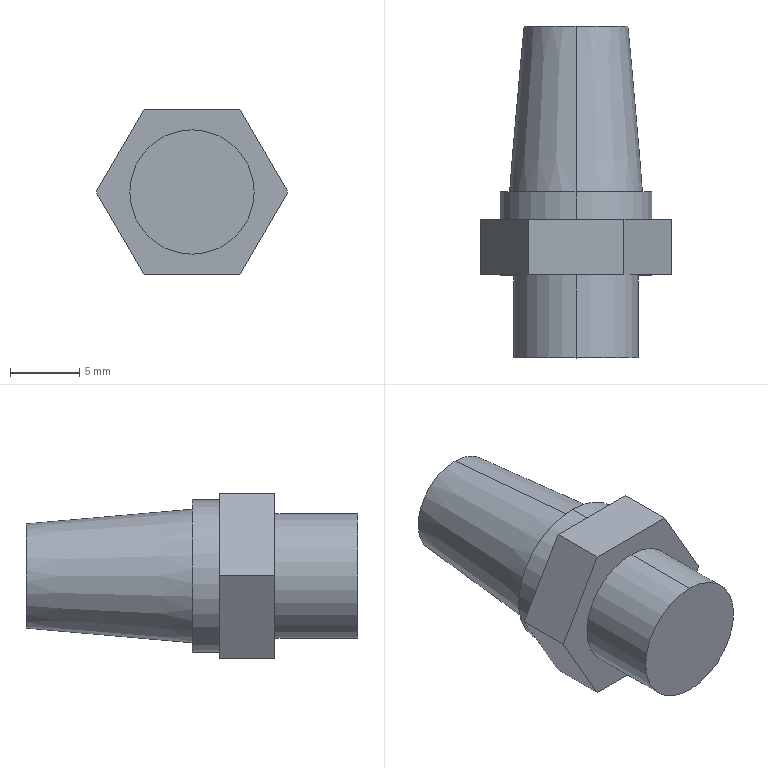Part | STEP file | Universal Copper Muffler BSL-01 | 1 solid | 17 faces | box 13.856 x 24 x 12 mm | volume 1771 mm3 | plane 11 | cylinder 4 | cone 2 | commonest cylinder face diameters 9 x2 11 x2
STEP:
#1=CARTESIAN_POINT('',(0.,0.,0.));
#2=DIRECTION('',(0.,0.,1.));
#3=DIRECTION('',(1.,0.,0.));
#4=AXIS2_PLACEMENT_3D('',#1,#2,#3);
#5=CARTESIAN_POINT('',(0.,24.,3.775));
#6=VERTEX_POINT('',#5);
#7=CARTESIAN_POINT('',(0.,24.,-3.775));
#8=VERTEX_POINT('',#7);
#9=CARTESIAN_POINT('',(0.,24.,0.));
#10=DIRECTION('',(0.,1.,0.));
#11=DIRECTION('',(0.,0.,1.));
#12=AXIS2_PLACEMENT_3D('',#9,#10,#11);
#13=CIRCLE('',#12,3.775);
#14=CARTESIAN_POINT('',(0.,24.,0.));
#15=DIRECTION('',(0.,-1.,0.));
#16=DIRECTION('',(0.,0.,-1.));
#17=AXIS2_PLACEMENT_3D('',#14,#15,#16);
#18=CONICAL_SURFACE('',#17,3.775,0.08727);
#19=CARTESIAN_POINT('',(3.142,0.));
#20=DIRECTION('',(-1.,0.));
#21=VECTOR('',#20,1.);
#22=LINE('',#19,#21);
#23=(GEOMETRIC_REPRESENTATION_CONTEXT(2)PARAMETRIC_REPRESENTATION_CONTEXT()REPRESENTATION_CONTEXT('',''));
#24=DEFINITIONAL_REPRESENTATION('',(#22),#23);
#25=PCURVE('',#18,#24);
#26=CARTESIAN_POINT('',(0.,24.,0.));
#27=DIRECTION('',(0.,1.,0.));
#28=DIRECTION('',(0.,0.,1.));
#29=AXIS2_PLACEMENT_3D('',#26,#27,#28);
#30=PLANE('',#29);
#31=CARTESIAN_POINT('',(0.,0.));
#32=DIRECTION('',(1.,0.));
#33=AXIS2_PLACEMENT_2D('',#31,#32);
#34=CIRCLE('',#33,3.775);
#35=(GEOMETRIC_REPRESENTATION_CONTEXT(2)PARAMETRIC_REPRESENTATION_CONTEXT()REPRESENTATION_CONTEXT('',''));
#36=DEFINITIONAL_REPRESENTATION('',(#34),#35);
#37=PCURVE('',#30,#36);
#38=SURFACE_CURVE('',#13,(#25,#37),.PCURVE_S1.);
#39=EDGE_CURVE('',#6,#8,#38,.T.);
#40=ORIENTED_EDGE('',*,*,#39,.F.);
#41=CARTESIAN_POINT('',(0.,12.,4.825));
#42=VERTEX_POINT('',#41);
#43=CARTESIAN_POINT('',(0.,24.,3.775));
#44=DIRECTION('',(0.,-0.9962,0.08716));
#45=VECTOR('',#44,1.);
#46=LINE('',#43,#45);
#47=CARTESIAN_POINT('',(3.142,0.));
#48=DIRECTION('',(0.,1.));
#49=VECTOR('',#48,1.);
#50=LINE('',#47,#49);
#51=(GEOMETRIC_REPRESENTATION_CONTEXT(2)PARAMETRIC_REPRESENTATION_CONTEXT()REPRESENTATION_CONTEXT('',''));
#52=DEFINITIONAL_REPRESENTATION('',(#50),#51);
#53=PCURVE('',#18,#52);
#54=CARTESIAN_POINT('',(0.,24.,0.));
#55=DIRECTION('',(0.,-1.,0.));
#56=DIRECTION('',(0.,0.,-1.));
#57=AXIS2_PLACEMENT_3D('',#54,#55,#56);
#58=CONICAL_SURFACE('',#57,3.775,0.08727);
#59=CARTESIAN_POINT('',(3.142,0.));
#60=DIRECTION('',(0.,1.));
#61=VECTOR('',#60,1.);
#62=LINE('',#59,#61);
#63=(GEOMETRIC_REPRESENTATION_CONTEXT(2)PARAMETRIC_REPRESENTATION_CONTEXT()REPRESENTATION_CONTEXT('',''));
#64=DEFINITIONAL_REPRESENTATION('',(#62),#63);
#65=PCURVE('',#58,#64);
#66=SURFACE_CURVE('',#46,(#53,#65),.PCURVE_S1.);
#67=EDGE_CURVE('',#6,#42,#66,.T.);
#68=ORIENTED_EDGE('',*,*,#67,.T.);
#69=CARTESIAN_POINT('',(0.,12.,-4.825));
#70=VERTEX_POINT('',#69);
#71=CARTESIAN_POINT('',(0.,12.,0.));
#72=DIRECTION('',(0.,-1.,0.));
#73=DIRECTION('',(0.,0.,1.));
#74=AXIS2_PLACEMENT_3D('',#71,#72,#73);
#75=CIRCLE('',#74,4.825);
#76=CARTESIAN_POINT('',(-3.142,12.));
#77=DIRECTION('',(1.,0.));
#78=VECTOR('',#77,1.);
#79=LINE('',#76,#78);
#80=(GEOMETRIC_REPRESENTATION_CONTEXT(2)PARAMETRIC_REPRESENTATION_CONTEXT()REPRESENTATION_CONTEXT('',''));
#81=DEFINITIONAL_REPRESENTATION('',(#79),#80);
#82=PCURVE('',#18,#81);
#83=CARTESIAN_POINT('',(0.,12.,0.));
#84=DIRECTION('',(0.,1.,0.));
#85=DIRECTION('',(0.,0.,1.));
#86=AXIS2_PLACEMENT_3D('',#83,#84,#85);
#87=PLANE('',#86);
#88=CARTESIAN_POINT('',(4.825,0.));
#89=CARTESIAN_POINT('',(4.825,-8.357));
#90=CARTESIAN_POINT('',(-2.413,-4.179));
#91=CARTESIAN_POINT('',(-9.65,0.));
#92=CARTESIAN_POINT('',(-2.413,4.179));
#93=CARTESIAN_POINT('',(4.825,8.357));
#94=CARTESIAN_POINT('',(4.825,0.));
#95=(BOUNDED_CURVE()B_SPLINE_CURVE(2,(#88,#89,#90,#91,#92,#93,#94),.UNSPECIFIED.,.T.,.F.)B_SPLINE_CURVE_WITH_KNOTS((1,2,2,2,2,1),(-2.094,0.,2.094,4.189,6.283,8.378),.UNSPECIFIED.)CURVE()GEOMETRIC_REPRESENTATION_ITEM()RATIONAL_B_SPLINE_CURVE((1.,0.5,1.,0.5,1.,0.5,1.))REPRESENTATION_ITEM(''));
#96=(GEOMETRIC_REPRESENTATION_CONTEXT(2)PARAMETRIC_REPRESENTATION_CONTEXT()REPRESENTATION_CONTEXT('',''));
#97=DEFINITIONAL_REPRESENTATION('',(#95),#96);
#98=PCURVE('',#87,#97);
#99=SURFACE_CURVE('',#75,(#82,#98),.PCURVE_S1.);
#100=EDGE_CURVE('',#70,#42,#99,.T.);
#101=ORIENTED_EDGE('',*,*,#100,.F.);
#102=CARTESIAN_POINT('',(0.,24.,-3.775));
#103=DIRECTION('',(0.,-0.9962,-0.08716));
#104=VECTOR('',#103,1.);
#105=LINE('',#102,#104);
#106=CARTESIAN_POINT('',(0.,0.));
#107=DIRECTION('',(0.,1.));
#108=VECTOR('',#107,1.);
#109=LINE('',#106,#108);
#110=(GEOMETRIC_REPRESENTATION_CONTEXT(2)PARAMETRIC_REPRESENTATION_CONTEXT()REPRESENTATION_CONTEXT('',''));
#111=DEFINITIONAL_REPRESENTATION('',(#109),#110);
#112=PCURVE('',#18,#111);
#113=CARTESIAN_POINT('',(6.283,0.));
#114=DIRECTION('',(0.,1.));
#115=VECTOR('',#114,1.);
#116=LINE('',#113,#115);
#117=(GEOMETRIC_REPRESENTATION_CONTEXT(2)PARAMETRIC_REPRESENTATION_CONTEXT()REPRESENTATION_CONTEXT('',''));
#118=DEFINITIONAL_REPRESENTATION('',(#116),#117);
#119=PCURVE('',#58,#118);
#120=SURFACE_CURVE('',#105,(#112,#119),.PCURVE_S1.);
#121=EDGE_CURVE('',#8,#70,#120,.T.);
#122=ORIENTED_EDGE('',*,*,#121,.F.);
#123=EDGE_LOOP('',(#40,#68,#101,#122));
#124=FACE_BOUND('',#123,.T.);
#125=ADVANCED_FACE('',(#124),#18,.T.);
#126=CARTESIAN_POINT('',(0.,12.,5.5));
#127=VERTEX_POINT('',#126);
#128=CARTESIAN_POINT('',(0.,12.,-5.5));
#129=VERTEX_POINT('',#128);
#130=CARTESIAN_POINT('',(0.,12.,0.));
#131=DIRECTION('',(0.,1.,0.));
#132=DIRECTION('',(0.,0.,1.));
#133=AXIS2_PLACEMENT_3D('',#130,#131,#132);
#134=CIRCLE('',#133,5.5);
#135=CARTESIAN_POINT('',(0.,12.,0.));
#136=DIRECTION('',(0.,-1.,0.));
#137=DIRECTION('',(0.,0.,-1.));
#138=AXIS2_PLACEMENT_3D('',#135,#136,#137);
#139=CYLINDRICAL_SURFACE('',#138,5.5);
#140=CARTESIAN_POINT('',(3.142,0.));
#141=DIRECTION('',(-1.,0.));
#142=VECTOR('',#141,1.);
#143=LINE('',#140,#142);
#144=(GEOMETRIC_REPRESENTATION_CONTEXT(2)PARAMETRIC_REPRESENTATION_CONTEXT()REPRESENTATION_CONTEXT('',''));
#145=DEFINITIONAL_REPRESENTATION('',(#143),#144);
#146=PCURVE('',#139,#145);
#147=CARTESIAN_POINT('',(0.,0.));
#148=DIRECTION('',(1.,0.));
#149=AXIS2_PLACEMENT_2D('',#147,#148);
#150=CIRCLE('',#149,5.5);
#151=(GEOMETRIC_REPRESENTATION_CONTEXT(2)PARAMETRIC_REPRESENTATION_CONTEXT()REPRESENTATION_CONTEXT('',''));
#152=DEFINITIONAL_REPRESENTATION('',(#150),#151);
#153=PCURVE('',#87,#152);
#154=SURFACE_CURVE('',#134,(#146,#153),.PCURVE_S1.);
#155=EDGE_CURVE('',#127,#129,#154,.T.);
#156=ORIENTED_EDGE('',*,*,#155,.F.);
#157=CARTESIAN_POINT('',(0.,10.,5.5));
#158=VERTEX_POINT('',#157);
#159=CARTESIAN_POINT('',(0.,12.,5.5));
#160=DIRECTION('',(0.,-1.,0.));
#161=VECTOR('',#160,1.);
#162=LINE('',#159,#161);
#163=CARTESIAN_POINT('',(3.142,0.));
#164=DIRECTION('',(0.,1.));
#165=VECTOR('',#164,1.);
#166=LINE('',#163,#165);
#167=(GEOMETRIC_REPRESENTATION_CONTEXT(2)PARAMETRIC_REPRESENTATION_CONTEXT()REPRESENTATION_CONTEXT('',''));
#168=DEFINITIONAL_REPRESENTATION('',(#166),#167);
#169=PCURVE('',#139,#168);
#170=CARTESIAN_POINT('',(0.,12.,0.));
#171=DIRECTION('',(0.,-1.,0.));
#172=DIRECTION('',(0.,0.,-1.));
#173=AXIS2_PLACEMENT_3D('',#170,#171,#172);
#174=CYLINDRICAL_SURFACE('',#173,5.5);
#175=CARTESIAN_POINT('',(3.142,0.));
#176=DIRECTION('',(0.,1.));
#177=VECTOR('',#176,1.);
#178=LINE('',#175,#177);
#179=(GEOMETRIC_REPRESENTATION_CONTEXT(2)PARAMETRIC_REPRESENTATION_CONTEXT()REPRESENTATION_CONTEXT('',''));
#180=DEFINITIONAL_REPRESENTATION('',(#178),#179);
#181=PCURVE('',#174,#180);
#182=SURFACE_CURVE('',#162,(#169,#181),.PCURVE_S1.);
#183=EDGE_CURVE('',#127,#158,#182,.T.);
#184=ORIENTED_EDGE('',*,*,#183,.T.);
#185=CARTESIAN_POINT('',(0.,10.,-5.5));
#186=VERTEX_POINT('',#185);
#187=CARTESIAN_POINT('',(0.,10.,0.));
#188=DIRECTION('',(0.,1.,0.));
#189=DIRECTION('',(0.,0.,1.));
#190=AXIS2_PLACEMENT_3D('',#187,#188,#189);
#191=CIRCLE('',#190,5.5);
#192=CARTESIAN_POINT('',(3.142,2.));
#193=DIRECTION('',(-1.,0.));
#194=VECTOR('',#193,1.);
#195=LINE('',#192,#194);
#196=(GEOMETRIC_REPRESENTATION_CONTEXT(2)PARAMETRIC_REPRESENTATION_CONTEXT()REPRESENTATION_CONTEXT('',''));
#197=DEFINITIONAL_REPRESENTATION('',(#195),#196);
#198=PCURVE('',#139,#197);
#199=CARTESIAN_POINT('',(0.,10.,0.));
#200=DIRECTION('',(0.,1.,0.));
#201=DIRECTION('',(0.,0.,1.));
#202=AXIS2_PLACEMENT_3D('',#199,#200,#201);
#203=PLANE('',#202);
#204=CARTESIAN_POINT('',(0.,0.));
#205=DIRECTION('',(1.,0.));
#206=AXIS2_PLACEMENT_2D('',#204,#205);
#207=CIRCLE('',#206,5.5);
#208=(GEOMETRIC_REPRESENTATION_CONTEXT(2)PARAMETRIC_REPRESENTATION_CONTEXT()REPRESENTATION_CONTEXT('',''));
#209=DEFINITIONAL_REPRESENTATION('',(#207),#208);
#210=PCURVE('',#203,#209);
#211=SURFACE_CURVE('',#191,(#198,#210),.PCURVE_S1.);
#212=EDGE_CURVE('',#158,#186,#211,.T.);
#213=ORIENTED_EDGE('',*,*,#212,.T.);
#214=CARTESIAN_POINT('',(0.,12.,-5.5));
#215=DIRECTION('',(0.,-1.,0.));
#216=VECTOR('',#215,1.);
#217=LINE('',#214,#216);
#218=CARTESIAN_POINT('',(0.,0.));
#219=DIRECTION('',(0.,1.));
#220=VECTOR('',#219,1.);
#221=LINE('',#218,#220);
#222=(GEOMETRIC_REPRESENTATION_CONTEXT(2)PARAMETRIC_REPRESENTATION_CONTEXT()REPRESENTATION_CONTEXT('',''));
#223=DEFINITIONAL_REPRESENTATION('',(#221),#222);
#224=PCURVE('',#139,#223);
#225=CARTESIAN_POINT('',(6.283,0.));
#226=DIRECTION('',(0.,1.));
#227=VECTOR('',#226,1.);
#228=LINE('',#225,#227);
#229=(GEOMETRIC_REPRESENTATION_CONTEXT(2)PARAMETRIC_REPRESENTATION_CONTEXT()REPRESENTATION_CONTEXT('',''));
#230=DEFINITIONAL_REPRESENTATION('',(#228),#229);
#231=PCURVE('',#174,#230);
#232=SURFACE_CURVE('',#217,(#224,#231),.PCURVE_S1.);
#233=EDGE_CURVE('',#129,#186,#232,.T.);
#234=ORIENTED_EDGE('',*,*,#233,.F.);
#235=EDGE_LOOP('',(#156,#184,#213,#234));
#236=FACE_BOUND('',#235,.T.);
#237=ADVANCED_FACE('',(#236),#139,.T.);
#238=CARTESIAN_POINT('',(0.,6.,4.5));
#239=VERTEX_POINT('',#238);
#240=CARTESIAN_POINT('',(0.,6.,-4.5));
#241=VERTEX_POINT('',#240);
#242=CARTESIAN_POINT('',(0.,6.,0.));
#243=DIRECTION('',(0.,1.,0.));
#244=DIRECTION('',(0.,0.,1.));
#245=AXIS2_PLACEMENT_3D('',#242,#243,#244);
#246=CIRCLE('',#245,4.5);
#247=CARTESIAN_POINT('',(0.,6.,0.));
#248=DIRECTION('',(0.,-1.,0.));
#249=DIRECTION('',(0.,0.,-1.));
#250=AXIS2_PLACEMENT_3D('',#247,#248,#249);
#251=CYLINDRICAL_SURFACE('',#250,4.5);
#252=CARTESIAN_POINT('',(3.142,0.));
#253=DIRECTION('',(-1.,0.));
#254=VECTOR('',#253,1.);
#255=LINE('',#252,#254);
#256=(GEOMETRIC_REPRESENTATION_CONTEXT(2)PARAMETRIC_REPRESENTATION_CONTEXT()REPRESENTATION_CONTEXT('',''));
#257=DEFINITIONAL_REPRESENTATION('',(#255),#256);
#258=PCURVE('',#251,#257);
#259=CARTESIAN_POINT('',(0.,6.,0.));
#260=DIRECTION('',(0.,1.,0.));
#261=DIRECTION('',(0.,0.,1.));
#262=AXIS2_PLACEMENT_3D('',#259,#260,#261);
#263=PLANE('',#262);
#264=CARTESIAN_POINT('',(0.,0.));
#265=DIRECTION('',(1.,0.));
#266=AXIS2_PLACEMENT_2D('',#264,#265);
#267=CIRCLE('',#266,4.5);
#268=(GEOMETRIC_REPRESENTATION_CONTEXT(2)PARAMETRIC_REPRESENTATION_CONTEXT()REPRESENTATION_CONTEXT('',''));
#269=DEFINITIONAL_REPRESENTATION('',(#267),#268);
#270=PCURVE('',#263,#269);
#271=SURFACE_CURVE('',#246,(#258,#270),.PCURVE_S1.);
#272=EDGE_CURVE('',#239,#241,#271,.T.);
#273=ORIENTED_EDGE('',*,*,#272,.F.);
#274=CARTESIAN_POINT('',(0.,0.,4.5));
#275=VERTEX_POINT('',#274);
#276=CARTESIAN_POINT('',(0.,6.,4.5));
#277=DIRECTION('',(0.,-1.,0.));
#278=VECTOR('',#277,1.);
#279=LINE('',#276,#278);
#280=CARTESIAN_POINT('',(3.142,0.));
#281=DIRECTION('',(0.,1.));
#282=VECTOR('',#281,1.);
#283=LINE('',#280,#282);
#284=(GEOMETRIC_REPRESENTATION_CONTEXT(2)PARAMETRIC_REPRESENTATION_CONTEXT()REPRESENTATION_CONTEXT('',''));
#285=DEFINITIONAL_REPRESENTATION('',(#283),#284);
#286=PCURVE('',#251,#285);
#287=CARTESIAN_POINT('',(0.,6.,0.));
#288=DIRECTION('',(0.,-1.,0.));
#289=DIRECTION('',(0.,0.,-1.));
#290=AXIS2_PLACEMENT_3D('',#287,#288,#289);
#291=CYLINDRICAL_SURFACE('',#290,4.5);
#292=CARTESIAN_POINT('',(3.142,0.));
#293=DIRECTION('',(0.,1.));
#294=VECTOR('',#293,1.);
#295=LINE('',#292,#294);
#296=(GEOMETRIC_REPRESENTATION_CONTEXT(2)PARAMETRIC_REPRESENTATION_CONTEXT()REPRESENTATION_CONTEXT('',''));
#297=DEFINITIONAL_REPRESENTATION('',(#295),#296);
#298=PCURVE('',#291,#297);
#299=SURFACE_CURVE('',#279,(#286,#298),.PCURVE_S1.);
#300=EDGE_CURVE('',#239,#275,#299,.T.);
#301=ORIENTED_EDGE('',*,*,#300,.T.);
#302=CARTESIAN_POINT('',(0.,0.,-4.5));
#303=VERTEX_POINT('',#302);
#304=CARTESIAN_POINT('',(0.,0.,0.));
#305=DIRECTION('',(0.,1.,0.));
#306=DIRECTION('',(0.,0.,1.));
#307=AXIS2_PLACEMENT_3D('',#304,#305,#306);
#308=CIRCLE('',#307,4.5);
#309=CARTESIAN_POINT('',(3.142,6.));
#310=DIRECTION('',(-1.,0.));
#311=VECTOR('',#310,1.);
#312=LINE('',#309,#311);
#313=(GEOMETRIC_REPRESENTATION_CONTEXT(2)PARAMETRIC_REPRESENTATION_CONTEXT()REPRESENTATION_CONTEXT('',''));
#314=DEFINITIONAL_REPRESENTATION('',(#312),#313);
#315=PCURVE('',#251,#314);
#316=CARTESIAN_POINT('',(0.,0.,0.));
#317=DIRECTION('',(0.,1.,0.));
#318=DIRECTION('',(0.,0.,1.));
#319=AXIS2_PLACEMENT_3D('',#316,#317,#318);
#320=PLANE('',#319);
#321=CARTESIAN_POINT('',(0.,0.));
#322=DIRECTION('',(1.,0.));
#323=AXIS2_PLACEMENT_2D('',#321,#322);
#324=CIRCLE('',#323,4.5);
#325=(GEOMETRIC_REPRESENTATION_CONTEXT(2)PARAMETRIC_REPRESENTATION_CONTEXT()REPRESENTATION_CONTEXT('',''));
#326=DEFINITIONAL_REPRESENTATION('',(#324),#325);
#327=PCURVE('',#320,#326);
#328=SURFACE_CURVE('',#308,(#315,#327),.PCURVE_S1.);
#329=EDGE_CURVE('',#275,#303,#328,.T.);
#330=ORIENTED_EDGE('',*,*,#329,.T.);
#331=CARTESIAN_POINT('',(0.,6.,-4.5));
#332=DIRECTION('',(0.,-1.,0.));
#333=VECTOR('',#332,1.);
#334=LINE('',#331,#333);
#335=CARTESIAN_POINT('',(0.,0.));
#336=DIRECTION('',(0.,1.));
#337=VECTOR('',#336,1.);
#338=LINE('',#335,#337);
#339=(GEOMETRIC_REPRESENTATION_CONTEXT(2)PARAMETRIC_REPRESENTATION_CONTEXT()REPRESENTATION_CONTEXT('',''));
#340=DEFINITIONAL_REPRESENTATION('',(#338),#339);
#341=PCURVE('',#251,#340);
#342=CARTESIAN_POINT('',(6.283,0.));
#343=DIRECTION('',(0.,1.));
#344=VECTOR('',#343,1.);
#345=LINE('',#342,#344);
#346=(GEOMETRIC_REPRESENTATION_CONTEXT(2)PARAMETRIC_REPRESENTATION_CONTEXT()REPRESENTATION_CONTEXT('',''));
#347=DEFINITIONAL_REPRESENTATION('',(#345),#346);
#348=PCURVE('',#291,#347);
#349=SURFACE_CURVE('',#334,(#341,#348),.PCURVE_S1.);
#350=EDGE_CURVE('',#241,#303,#349,.T.);
#351=ORIENTED_EDGE('',*,*,#350,.F.);
#352=EDGE_LOOP('',(#273,#301,#330,#351));
#353=FACE_BOUND('',#352,.T.);
#354=ADVANCED_FACE('',(#353),#251,.T.);
#355=ORIENTED_EDGE('',*,*,#300,.F.);
#356=CARTESIAN_POINT('',(0.,6.,0.));
#357=DIRECTION('',(0.,1.,0.));
#358=DIRECTION('',(0.,0.,1.));
#359=AXIS2_PLACEMENT_3D('',#356,#357,#358);
#360=CIRCLE('',#359,4.5);
#361=CARTESIAN_POINT('',(9.425,0.));
#362=DIRECTION('',(-1.,0.));
#363=VECTOR('',#362,1.);
#364=LINE('',#361,#363);
#365=(GEOMETRIC_REPRESENTATION_CONTEXT(2)PARAMETRIC_REPRESENTATION_CONTEXT()REPRESENTATION_CONTEXT('',''));
#366=DEFINITIONAL_REPRESENTATION('',(#364),#365);
#367=PCURVE('',#291,#366);
#368=CARTESIAN_POINT('',(0.,0.));
#369=DIRECTION('',(1.,0.));
#370=AXIS2_PLACEMENT_2D('',#368,#369);
#371=CIRCLE('',#370,4.5);
#372=(GEOMETRIC_REPRESENTATION_CONTEXT(2)PARAMETRIC_REPRESENTATION_CONTEXT()REPRESENTATION_CONTEXT('',''));
#373=DEFINITIONAL_REPRESENTATION('',(#371),#372);
#374=PCURVE('',#263,#373);
#375=SURFACE_CURVE('',#360,(#367,#374),.PCURVE_S1.);
#376=EDGE_CURVE('',#241,#239,#375,.T.);
#377=ORIENTED_EDGE('',*,*,#376,.F.);
#378=ORIENTED_EDGE('',*,*,#350,.T.);
#379=CARTESIAN_POINT('',(0.,0.,0.));
#380=DIRECTION('',(0.,1.,0.));
#381=DIRECTION('',(0.,0.,1.));
#382=AXIS2_PLACEMENT_3D('',#379,#380,#381);
#383=CIRCLE('',#382,4.5);
#384=CARTESIAN_POINT('',(9.425,6.));
#385=DIRECTION('',(-1.,0.));
#386=VECTOR('',#385,1.);
#387=LINE('',#384,#386);
#388=(GEOMETRIC_REPRESENTATION_CONTEXT(2)PARAMETRIC_REPRESENTATION_CONTEXT()REPRESENTATION_CONTEXT('',''));
#389=DEFINITIONAL_REPRESENTATION('',(#387),#388);
#390=PCURVE('',#291,#389);
#391=CARTESIAN_POINT('',(0.,0.));
#392=DIRECTION('',(1.,0.));
#393=AXIS2_PLACEMENT_2D('',#391,#392);
#394=CIRCLE('',#393,4.5);
#395=(GEOMETRIC_REPRESENTATION_CONTEXT(2)PARAMETRIC_REPRESENTATION_CONTEXT()REPRESENTATION_CONTEXT('',''));
#396=DEFINITIONAL_REPRESENTATION('',(#394),#395);
#397=PCURVE('',#320,#396);
#398=SURFACE_CURVE('',#383,(#390,#397),.PCURVE_S1.);
#399=EDGE_CURVE('',#303,#275,#398,.T.);
#400=ORIENTED_EDGE('',*,*,#399,.T.);
#401=EDGE_LOOP('',(#355,#377,#378,#400));
#402=FACE_BOUND('',#401,.T.);
#403=ADVANCED_FACE('',(#402),#291,.T.);
#404=ORIENTED_EDGE('',*,*,#399,.F.);
#405=ORIENTED_EDGE('',*,*,#329,.F.);
#406=EDGE_LOOP('',(#404,#405));
#407=FACE_BOUND('',#406,.T.);
#408=ADVANCED_FACE('',(#407),#320,.F.);
#409=CARTESIAN_POINT('',(3.464,6.,6.));
#410=VERTEX_POINT('',#409);
#411=CARTESIAN_POINT('',(6.928,6.,0.));
#412=VERTEX_POINT('',#411);
#413=CARTESIAN_POINT('',(3.464,6.,6.));
#414=DIRECTION('',(0.5,0.,-0.866));
#415=VECTOR('',#414,1.);
#416=LINE('',#413,#415);
#417=CARTESIAN_POINT('',(3.464,10.,6.));
#418=DIRECTION('',(-0.866,0.,-0.5));
#419=DIRECTION('',(-0.5,0.,0.866));
#420=AXIS2_PLACEMENT_3D('',#417,#418,#419);
#421=PLANE('',#420);
#422=CARTESIAN_POINT('',(0.,-4.));
#423=DIRECTION('',(-1.,0.));
#424=VECTOR('',#423,1.);
#425=LINE('',#422,#424);
#426=(GEOMETRIC_REPRESENTATION_CONTEXT(2)PARAMETRIC_REPRESENTATION_CONTEXT()REPRESENTATION_CONTEXT('',''));
#427=DEFINITIONAL_REPRESENTATION('',(#425),#426);
#428=PCURVE('',#421,#427);
#429=CARTESIAN_POINT('',(6.,3.464));
#430=DIRECTION('',(-0.866,0.5));
#431=VECTOR('',#430,1.);
#432=LINE('',#429,#431);
#433=(GEOMETRIC_REPRESENTATION_CONTEXT(2)PARAMETRIC_REPRESENTATION_CONTEXT()REPRESENTATION_CONTEXT('',''));
#434=DEFINITIONAL_REPRESENTATION('',(#432),#433);
#435=PCURVE('',#263,#434);
#436=SURFACE_CURVE('',#416,(#428,#435),.PCURVE_S1.);
#437=EDGE_CURVE('',#410,#412,#436,.T.);
#438=ORIENTED_EDGE('',*,*,#437,.T.);
#439=CARTESIAN_POINT('',(6.928,10.,0.));
#440=VERTEX_POINT('',#439);
#441=CARTESIAN_POINT('',(6.928,10.,0.));
#442=DIRECTION('',(0.,-1.,0.));
#443=VECTOR('',#442,1.);
#444=LINE('',#441,#443);
#445=CARTESIAN_POINT('',(-6.928,0.));
#446=DIRECTION('',(0.,-1.));
#447=VECTOR('',#446,1.);
#448=LINE('',#445,#447);
#449=(GEOMETRIC_REPRESENTATION_CONTEXT(2)PARAMETRIC_REPRESENTATION_CONTEXT()REPRESENTATION_CONTEXT('',''));
#450=DEFINITIONAL_REPRESENTATION('',(#448),#449);
#451=PCURVE('',#421,#450);
#452=CARTESIAN_POINT('',(6.928,10.,0.));
#453=DIRECTION('',(-0.866,0.,0.5));
#454=DIRECTION('',(0.5,0.,0.866));
#455=AXIS2_PLACEMENT_3D('',#452,#453,#454);
#456=PLANE('',#455);
#457=CARTESIAN_POINT('',(0.,0.));
#458=DIRECTION('',(0.,-1.));
#459=VECTOR('',#458,1.);
#460=LINE('',#457,#459);
#461=(GEOMETRIC_REPRESENTATION_CONTEXT(2)PARAMETRIC_REPRESENTATION_CONTEXT()REPRESENTATION_CONTEXT('',''));
#462=DEFINITIONAL_REPRESENTATION('',(#460),#461);
#463=PCURVE('',#456,#462);
#464=SURFACE_CURVE('',#444,(#451,#463),.PCURVE_S1.);
#465=EDGE_CURVE('',#440,#412,#464,.T.);
#466=ORIENTED_EDGE('',*,*,#465,.F.);
#467=CARTESIAN_POINT('',(3.464,10.,6.));
#468=VERTEX_POINT('',#467);
#469=CARTESIAN_POINT('',(3.464,10.,6.));
#470=DIRECTION('',(0.5,0.,-0.866));
#471=VECTOR('',#470,1.);
#472=LINE('',#469,#471);
#473=CARTESIAN_POINT('',(0.,0.));
#474=DIRECTION('',(-1.,0.));
#475=VECTOR('',#474,1.);
#476=LINE('',#473,#475);
#477=(GEOMETRIC_REPRESENTATION_CONTEXT(2)PARAMETRIC_REPRESENTATION_CONTEXT()REPRESENTATION_CONTEXT('',''));
#478=DEFINITIONAL_REPRESENTATION('',(#476),#477);
#479=PCURVE('',#421,#478);
#480=CARTESIAN_POINT('',(6.,3.464));
#481=DIRECTION('',(-0.866,0.5));
#482=VECTOR('',#481,1.);
#483=LINE('',#480,#482);
#484=(GEOMETRIC_REPRESENTATION_CONTEXT(2)PARAMETRIC_REPRESENTATION_CONTEXT()REPRESENTATION_CONTEXT('',''));
#485=DEFINITIONAL_REPRESENTATION('',(#483),#484);
#486=PCURVE('',#203,#485);
#487=SURFACE_CURVE('',#472,(#479,#486),.PCURVE_S1.);
#488=EDGE_CURVE('',#468,#440,#487,.T.);
#489=ORIENTED_EDGE('',*,*,#488,.F.);
#490=CARTESIAN_POINT('',(3.464,10.,6.));
#491=DIRECTION('',(0.,-1.,0.));
#492=VECTOR('',#491,1.);
#493=LINE('',#490,#492);
#494=CARTESIAN_POINT('',(0.,0.));
#495=DIRECTION('',(0.,-1.));
#496=VECTOR('',#495,1.);
#497=LINE('',#494,#496);
#498=(GEOMETRIC_REPRESENTATION_CONTEXT(2)PARAMETRIC_REPRESENTATION_CONTEXT()REPRESENTATION_CONTEXT('',''));
#499=DEFINITIONAL_REPRESENTATION('',(#497),#498);
#500=PCURVE('',#421,#499);
#501=CARTESIAN_POINT('',(-3.464,10.,6.));
#502=DIRECTION('',(0.,0.,-1.));
#503=DIRECTION('',(-1.,0.,0.));
#504=AXIS2_PLACEMENT_3D('',#501,#502,#503);
#505=PLANE('',#504);
#506=CARTESIAN_POINT('',(-6.928,0.));
#507=DIRECTION('',(0.,-1.));
#508=VECTOR('',#507,1.);
#509=LINE('',#506,#508);
#510=(GEOMETRIC_REPRESENTATION_CONTEXT(2)PARAMETRIC_REPRESENTATION_CONTEXT()REPRESENTATION_CONTEXT('',''));
#511=DEFINITIONAL_REPRESENTATION('',(#509),#510);
#512=PCURVE('',#505,#511);
#513=SURFACE_CURVE('',#493,(#500,#512),.PCURVE_S1.);
#514=EDGE_CURVE('',#468,#410,#513,.T.);
#515=ORIENTED_EDGE('',*,*,#514,.T.);
#516=EDGE_LOOP('',(#438,#466,#489,#515));
#517=FACE_BOUND('',#516,.T.);
#518=ADVANCED_FACE('',(#517),#421,.F.);
#519=CARTESIAN_POINT('',(3.464,6.,-6.));
#520=VERTEX_POINT('',#519);
#521=CARTESIAN_POINT('',(6.928,6.,0.));
#522=DIRECTION('',(-0.5,0.,-0.866));
#523=VECTOR('',#522,1.);
#524=LINE('',#521,#523);
#525=CARTESIAN_POINT('',(0.,-4.));
#526=DIRECTION('',(-1.,0.));
#527=VECTOR('',#526,1.);
#528=LINE('',#525,#527);
#529=(GEOMETRIC_REPRESENTATION_CONTEXT(2)PARAMETRIC_REPRESENTATION_CONTEXT()REPRESENTATION_CONTEXT('',''));
#530=DEFINITIONAL_REPRESENTATION('',(#528),#529);
#531=PCURVE('',#456,#530);
#532=CARTESIAN_POINT('',(0.,6.928));
#533=DIRECTION('',(-0.866,-0.5));
#534=VECTOR('',#533,1.);
#535=LINE('',#532,#534);
#536=(GEOMETRIC_REPRESENTATION_CONTEXT(2)PARAMETRIC_REPRESENTATION_CONTEXT()REPRESENTATION_CONTEXT('',''));
#537=DEFINITIONAL_REPRESENTATION('',(#535),#536);
#538=PCURVE('',#263,#537);
#539=SURFACE_CURVE('',#524,(#531,#538),.PCURVE_S1.);
#540=EDGE_CURVE('',#412,#520,#539,.T.);
#541=ORIENTED_EDGE('',*,*,#540,.T.);
#542=CARTESIAN_POINT('',(3.464,10.,-6.));
#543=VERTEX_POINT('',#542);
#544=CARTESIAN_POINT('',(3.464,10.,-6.));
#545=DIRECTION('',(0.,-1.,0.));
#546=VECTOR('',#545,1.);
#547=LINE('',#544,#546);
#548=CARTESIAN_POINT('',(-6.928,0.));
#549=DIRECTION('',(0.,-1.));
#550=VECTOR('',#549,1.);
#551=LINE('',#548,#550);
#552=(GEOMETRIC_REPRESENTATION_CONTEXT(2)PARAMETRIC_REPRESENTATION_CONTEXT()REPRESENTATION_CONTEXT('',''));
#553=DEFINITIONAL_REPRESENTATION('',(#551),#552);
#554=PCURVE('',#456,#553);
#555=CARTESIAN_POINT('',(3.464,10.,-6.));
#556=DIRECTION('',(0.,0.,1.));
#557=DIRECTION('',(1.,0.,0.));
#558=AXIS2_PLACEMENT_3D('',#555,#556,#557);
#559=PLANE('',#558);
#560=CARTESIAN_POINT('',(0.,0.));
#561=DIRECTION('',(0.,-1.));
#562=VECTOR('',#561,1.);
#563=LINE('',#560,#562);
#564=(GEOMETRIC_REPRESENTATION_CONTEXT(2)PARAMETRIC_REPRESENTATION_CONTEXT()REPRESENTATION_CONTEXT('',''));
#565=DEFINITIONAL_REPRESENTATION('',(#563),#564);
#566=PCURVE('',#559,#565);
#567=SURFACE_CURVE('',#547,(#554,#566),.PCURVE_S1.);
#568=EDGE_CURVE('',#543,#520,#567,.T.);
#569=ORIENTED_EDGE('',*,*,#568,.F.);
#570=CARTESIAN_POINT('',(6.928,10.,0.));
#571=DIRECTION('',(-0.5,0.,-0.866));
#572=VECTOR('',#571,1.);
#573=LINE('',#570,#572);
#574=CARTESIAN_POINT('',(0.,0.));
#575=DIRECTION('',(-1.,0.));
#576=VECTOR('',#575,1.);
#577=LINE('',#574,#576);
#578=(GEOMETRIC_REPRESENTATION_CONTEXT(2)PARAMETRIC_REPRESENTATION_CONTEXT()REPRESENTATION_CONTEXT('',''));
#579=DEFINITIONAL_REPRESENTATION('',(#577),#578);
#580=PCURVE('',#456,#579);
#581=CARTESIAN_POINT('',(0.,6.928));
#582=DIRECTION('',(-0.866,-0.5));
#583=VECTOR('',#582,1.);
#584=LINE('',#581,#583);
#585=(GEOMETRIC_REPRESENTATION_CONTEXT(2)PARAMETRIC_REPRESENTATION_CONTEXT()REPRESENTATION_CONTEXT('',''));
#586=DEFINITIONAL_REPRESENTATION('',(#584),#585);
#587=PCURVE('',#203,#586);
#588=SURFACE_CURVE('',#573,(#580,#587),.PCURVE_S1.);
#589=EDGE_CURVE('',#440,#543,#588,.T.);
#590=ORIENTED_EDGE('',*,*,#589,.F.);
#591=ORIENTED_EDGE('',*,*,#465,.T.);
#592=EDGE_LOOP('',(#541,#569,#590,#591));
#593=FACE_BOUND('',#592,.T.);
#594=ADVANCED_FACE('',(#593),#456,.F.);
#595=CARTESIAN_POINT('',(-3.464,6.,-6.));
#596=VERTEX_POINT('',#595);
#597=CARTESIAN_POINT('',(3.464,6.,-6.));
#598=DIRECTION('',(-1.,0.,0.));
#599=VECTOR('',#598,1.);
#600=LINE('',#597,#599);
#601=CARTESIAN_POINT('',(0.,-4.));
#602=DIRECTION('',(-1.,0.));
#603=VECTOR('',#602,1.);
#604=LINE('',#601,#603);
#605=(GEOMETRIC_REPRESENTATION_CONTEXT(2)PARAMETRIC_REPRESENTATION_CONTEXT()REPRESENTATION_CONTEXT('',''));
#606=DEFINITIONAL_REPRESENTATION('',(#604),#605);
#607=PCURVE('',#559,#606);
#608=CARTESIAN_POINT('',(-6.,3.464));
#609=DIRECTION('',(0.,-1.));
#610=VECTOR('',#609,1.);
#611=LINE('',#608,#610);
#612=(GEOMETRIC_REPRESENTATION_CONTEXT(2)PARAMETRIC_REPRESENTATION_CONTEXT()REPRESENTATION_CONTEXT('',''));
#613=DEFINITIONAL_REPRESENTATION('',(#611),#612);
#614=PCURVE('',#263,#613);
#615=SURFACE_CURVE('',#600,(#607,#614),.PCURVE_S1.);
#616=EDGE_CURVE('',#520,#596,#615,.T.);
#617=ORIENTED_EDGE('',*,*,#616,.T.);
#618=CARTESIAN_POINT('',(-3.464,10.,-6.));
#619=VERTEX_POINT('',#618);
#620=CARTESIAN_POINT('',(-3.464,10.,-6.));
#621=DIRECTION('',(0.,-1.,0.));
#622=VECTOR('',#621,1.);
#623=LINE('',#620,#622);
#624=CARTESIAN_POINT('',(-6.928,0.));
#625=DIRECTION('',(0.,-1.));
#626=VECTOR('',#625,1.);
#627=LINE('',#624,#626);
#628=(GEOMETRIC_REPRESENTATION_CONTEXT(2)PARAMETRIC_REPRESENTATION_CONTEXT()REPRESENTATION_CONTEXT('',''));
#629=DEFINITIONAL_REPRESENTATION('',(#627),#628);
#630=PCURVE('',#559,#629);
#631=CARTESIAN_POINT('',(-3.464,10.,-6.));
#632=DIRECTION('',(0.866,0.,0.5));
#633=DIRECTION('',(0.5,0.,-0.866));
#634=AXIS2_PLACEMENT_3D('',#631,#632,#633);
#635=PLANE('',#634);
#636=CARTESIAN_POINT('',(0.,0.));
#637=DIRECTION('',(0.,-1.));
#638=VECTOR('',#637,1.);
#639=LINE('',#636,#638);
#640=(GEOMETRIC_REPRESENTATION_CONTEXT(2)PARAMETRIC_REPRESENTATION_CONTEXT()REPRESENTATION_CONTEXT('',''));
#641=DEFINITIONAL_REPRESENTATION('',(#639),#640);
#642=PCURVE('',#635,#641);
#643=SURFACE_CURVE('',#623,(#630,#642),.PCURVE_S1.);
#644=EDGE_CURVE('',#619,#596,#643,.T.);
#645=ORIENTED_EDGE('',*,*,#644,.F.);
#646=CARTESIAN_POINT('',(3.464,10.,-6.));
#647=DIRECTION('',(-1.,0.,0.));
#648=VECTOR('',#647,1.);
#649=LINE('',#646,#648);
#650=CARTESIAN_POINT('',(0.,0.));
#651=DIRECTION('',(-1.,0.));
#652=VECTOR('',#651,1.);
#653=LINE('',#650,#652);
#654=(GEOMETRIC_REPRESENTATION_CONTEXT(2)PARAMETRIC_REPRESENTATION_CONTEXT()REPRESENTATION_CONTEXT('',''));
#655=DEFINITIONAL_REPRESENTATION('',(#653),#654);
#656=PCURVE('',#559,#655);
#657=CARTESIAN_POINT('',(-6.,3.464));
#658=DIRECTION('',(0.,-1.));
#659=VECTOR('',#658,1.);
#660=LINE('',#657,#659);
#661=(GEOMETRIC_REPRESENTATION_CONTEXT(2)PARAMETRIC_REPRESENTATION_CONTEXT()REPRESENTATION_CONTEXT('',''));
#662=DEFINITIONAL_REPRESENTATION('',(#660),#661);
#663=PCURVE('',#203,#662);
#664=SURFACE_CURVE('',#649,(#656,#663),.PCURVE_S1.);
#665=EDGE_CURVE('',#543,#619,#664,.T.);
#666=ORIENTED_EDGE('',*,*,#665,.F.);
#667=ORIENTED_EDGE('',*,*,#568,.T.);
#668=EDGE_LOOP('',(#617,#645,#666,#667));
#669=FACE_BOUND('',#668,.T.);
#670=ADVANCED_FACE('',(#669),#559,.F.);
#671=CARTESIAN_POINT('',(-6.928,6.,0.));
#672=VERTEX_POINT('',#671);
#673=CARTESIAN_POINT('',(-3.464,6.,-6.));
#674=DIRECTION('',(-0.5,0.,0.866));
#675=VECTOR('',#674,1.);
#676=LINE('',#673,#675);
#677=CARTESIAN_POINT('',(0.,-4.));
#678=DIRECTION('',(-1.,0.));
#679=VECTOR('',#678,1.);
#680=LINE('',#677,#679);
#681=(GEOMETRIC_REPRESENTATION_CONTEXT(2)PARAMETRIC_REPRESENTATION_CONTEXT()REPRESENTATION_CONTEXT('',''));
#682=DEFINITIONAL_REPRESENTATION('',(#680),#681);
#683=PCURVE('',#635,#682);
#684=CARTESIAN_POINT('',(-6.,-3.464));
#685=DIRECTION('',(0.866,-0.5));
#686=VECTOR('',#685,1.);
#687=LINE('',#684,#686);
#688=(GEOMETRIC_REPRESENTATION_CONTEXT(2)PARAMETRIC_REPRESENTATION_CONTEXT()REPRESENTATION_CONTEXT('',''));
#689=DEFINITIONAL_REPRESENTATION('',(#687),#688);
#690=PCURVE('',#263,#689);
#691=SURFACE_CURVE('',#676,(#683,#690),.PCURVE_S1.);
#692=EDGE_CURVE('',#596,#672,#691,.T.);
#693=ORIENTED_EDGE('',*,*,#692,.T.);
#694=CARTESIAN_POINT('',(-6.928,10.,0.));
#695=VERTEX_POINT('',#694);
#696=CARTESIAN_POINT('',(-6.928,10.,0.));
#697=DIRECTION('',(0.,-1.,0.));
#698=VECTOR('',#697,1.);
#699=LINE('',#696,#698);
#700=CARTESIAN_POINT('',(-6.928,0.));
#701=DIRECTION('',(0.,-1.));
#702=VECTOR('',#701,1.);
#703=LINE('',#700,#702);
#704=(GEOMETRIC_REPRESENTATION_CONTEXT(2)PARAMETRIC_REPRESENTATION_CONTEXT()REPRESENTATION_CONTEXT('',''));
#705=DEFINITIONAL_REPRESENTATION('',(#703),#704);
#706=PCURVE('',#635,#705);
#707=CARTESIAN_POINT('',(-6.928,10.,0.));
#708=DIRECTION('',(0.866,0.,-0.5));
#709=DIRECTION('',(-0.5,0.,-0.866));
#710=AXIS2_PLACEMENT_3D('',#707,#708,#709);
#711=PLANE('',#710);
#712=CARTESIAN_POINT('',(0.,0.));
#713=DIRECTION('',(0.,-1.));
#714=VECTOR('',#713,1.);
#715=LINE('',#712,#714);
#716=(GEOMETRIC_REPRESENTATION_CONTEXT(2)PARAMETRIC_REPRESENTATION_CONTEXT()REPRESENTATION_CONTEXT('',''));
#717=DEFINITIONAL_REPRESENTATION('',(#715),#716);
#718=PCURVE('',#711,#717);
#719=SURFACE_CURVE('',#699,(#706,#718),.PCURVE_S1.);
#720=EDGE_CURVE('',#695,#672,#719,.T.);
#721=ORIENTED_EDGE('',*,*,#720,.F.);
#722=CARTESIAN_POINT('',(-3.464,10.,-6.));
#723=DIRECTION('',(-0.5,0.,0.866));
#724=VECTOR('',#723,1.);
#725=LINE('',#722,#724);
#726=CARTESIAN_POINT('',(0.,0.));
#727=DIRECTION('',(-1.,0.));
#728=VECTOR('',#727,1.);
#729=LINE('',#726,#728);
#730=(GEOMETRIC_REPRESENTATION_CONTEXT(2)PARAMETRIC_REPRESENTATION_CONTEXT()REPRESENTATION_CONTEXT('',''));
#731=DEFINITIONAL_REPRESENTATION('',(#729),#730);
#732=PCURVE('',#635,#731);
#733=CARTESIAN_POINT('',(-6.,-3.464));
#734=DIRECTION('',(0.866,-0.5));
#735=VECTOR('',#734,1.);
#736=LINE('',#733,#735);
#737=(GEOMETRIC_REPRESENTATION_CONTEXT(2)PARAMETRIC_REPRESENTATION_CONTEXT()REPRESENTATION_CONTEXT('',''));
#738=DEFINITIONAL_REPRESENTATION('',(#736),#737);
#739=PCURVE('',#203,#738);
#740=SURFACE_CURVE('',#725,(#732,#739),.PCURVE_S1.);
#741=EDGE_CURVE('',#619,#695,#740,.T.);
#742=ORIENTED_EDGE('',*,*,#741,.F.);
#743=ORIENTED_EDGE('',*,*,#644,.T.);
#744=EDGE_LOOP('',(#693,#721,#742,#743));
#745=FACE_BOUND('',#744,.T.);
#746=ADVANCED_FACE('',(#745),#635,.F.);
#747=CARTESIAN_POINT('',(-3.464,6.,6.));
#748=VERTEX_POINT('',#747);
#749=CARTESIAN_POINT('',(-6.928,6.,0.));
#750=DIRECTION('',(0.5,0.,0.866));
#751=VECTOR('',#750,1.);
#752=LINE('',#749,#751);
#753=CARTESIAN_POINT('',(0.,-4.));
#754=DIRECTION('',(-1.,0.));
#755=VECTOR('',#754,1.);
#756=LINE('',#753,#755);
#757=(GEOMETRIC_REPRESENTATION_CONTEXT(2)PARAMETRIC_REPRESENTATION_CONTEXT()REPRESENTATION_CONTEXT('',''));
#758=DEFINITIONAL_REPRESENTATION('',(#756),#757);
#759=PCURVE('',#711,#758);
#760=CARTESIAN_POINT('',(0.,-6.928));
#761=DIRECTION('',(0.866,0.5));
#762=VECTOR('',#761,1.);
#763=LINE('',#760,#762);
#764=(GEOMETRIC_REPRESENTATION_CONTEXT(2)PARAMETRIC_REPRESENTATION_CONTEXT()REPRESENTATION_CONTEXT('',''));
#765=DEFINITIONAL_REPRESENTATION('',(#763),#764);
#766=PCURVE('',#263,#765);
#767=SURFACE_CURVE('',#752,(#759,#766),.PCURVE_S1.);
#768=EDGE_CURVE('',#672,#748,#767,.T.);
#769=ORIENTED_EDGE('',*,*,#768,.T.);
#770=CARTESIAN_POINT('',(-3.464,10.,6.));
#771=VERTEX_POINT('',#770);
#772=CARTESIAN_POINT('',(-3.464,10.,6.));
#773=DIRECTION('',(0.,-1.,0.));
#774=VECTOR('',#773,1.);
#775=LINE('',#772,#774);
#776=CARTESIAN_POINT('',(-6.928,0.));
#777=DIRECTION('',(0.,-1.));
#778=VECTOR('',#777,1.);
#779=LINE('',#776,#778);
#780=(GEOMETRIC_REPRESENTATION_CONTEXT(2)PARAMETRIC_REPRESENTATION_CONTEXT()REPRESENTATION_CONTEXT('',''));
#781=DEFINITIONAL_REPRESENTATION('',(#779),#780);
#782=PCURVE('',#711,#781);
#783=CARTESIAN_POINT('',(0.,0.));
#784=DIRECTION('',(0.,-1.));
#785=VECTOR('',#784,1.);
#786=LINE('',#783,#785);
#787=(GEOMETRIC_REPRESENTATION_CONTEXT(2)PARAMETRIC_REPRESENTATION_CONTEXT()REPRESENTATION_CONTEXT('',''));
#788=DEFINITIONAL_REPRESENTATION('',(#786),#787);
#789=PCURVE('',#505,#788);
#790=SURFACE_CURVE('',#775,(#782,#789),.PCURVE_S1.);
#791=EDGE_CURVE('',#771,#748,#790,.T.);
#792=ORIENTED_EDGE('',*,*,#791,.F.);
#793=CARTESIAN_POINT('',(-6.928,10.,0.));
#794=DIRECTION('',(0.5,0.,0.866));
#795=VECTOR('',#794,1.);
#796=LINE('',#793,#795);
#797=CARTESIAN_POINT('',(0.,0.));
#798=DIRECTION('',(-1.,0.));
#799=VECTOR('',#798,1.);
#800=LINE('',#797,#799);
#801=(GEOMETRIC_REPRESENTATION_CONTEXT(2)PARAMETRIC_REPRESENTATION_CONTEXT()REPRESENTATION_CONTEXT('',''));
#802=DEFINITIONAL_REPRESENTATION('',(#800),#801);
#803=PCURVE('',#711,#802);
#804=CARTESIAN_POINT('',(0.,-6.928));
#805=DIRECTION('',(0.866,0.5));
#806=VECTOR('',#805,1.);
#807=LINE('',#804,#806);
#808=(GEOMETRIC_REPRESENTATION_CONTEXT(2)PARAMETRIC_REPRESENTATION_CONTEXT()REPRESENTATION_CONTEXT('',''));
#809=DEFINITIONAL_REPRESENTATION('',(#807),#808);
#810=PCURVE('',#203,#809);
#811=SURFACE_CURVE('',#796,(#803,#810),.PCURVE_S1.);
#812=EDGE_CURVE('',#695,#771,#811,.T.);
#813=ORIENTED_EDGE('',*,*,#812,.F.);
#814=ORIENTED_EDGE('',*,*,#720,.T.);
#815=EDGE_LOOP('',(#769,#792,#813,#814));
#816=FACE_BOUND('',#815,.T.);
#817=ADVANCED_FACE('',(#816),#711,.F.);
#818=CARTESIAN_POINT('',(-3.464,6.,6.));
#819=DIRECTION('',(1.,0.,0.));
#820=VECTOR('',#819,1.);
#821=LINE('',#818,#820);
#822=CARTESIAN_POINT('',(0.,-4.));
#823=DIRECTION('',(-1.,0.));
#824=VECTOR('',#823,1.);
#825=LINE('',#822,#824);
#826=(GEOMETRIC_REPRESENTATION_CONTEXT(2)PARAMETRIC_REPRESENTATION_CONTEXT()REPRESENTATION_CONTEXT('',''));
#827=DEFINITIONAL_REPRESENTATION('',(#825),#826);
#828=PCURVE('',#505,#827);
#829=CARTESIAN_POINT('',(6.,-3.464));
#830=DIRECTION('',(0.,1.));
#831=VECTOR('',#830,1.);
#832=LINE('',#829,#831);
#833=(GEOMETRIC_REPRESENTATION_CONTEXT(2)PARAMETRIC_REPRESENTATION_CONTEXT()REPRESENTATION_CONTEXT('',''));
#834=DEFINITIONAL_REPRESENTATION('',(#832),#833);
#835=PCURVE('',#263,#834);
#836=SURFACE_CURVE('',#821,(#828,#835),.PCURVE_S1.);
#837=EDGE_CURVE('',#748,#410,#836,.T.);
#838=ORIENTED_EDGE('',*,*,#837,.T.);
#839=ORIENTED_EDGE('',*,*,#514,.F.);
#840=CARTESIAN_POINT('',(-3.464,10.,6.));
#841=DIRECTION('',(1.,0.,0.));
#842=VECTOR('',#841,1.);
#843=LINE('',#840,#842);
#844=CARTESIAN_POINT('',(0.,0.));
#845=DIRECTION('',(-1.,0.));
#846=VECTOR('',#845,1.);
#847=LINE('',#844,#846);
#848=(GEOMETRIC_REPRESENTATION_CONTEXT(2)PARAMETRIC_REPRESENTATION_CONTEXT()REPRESENTATION_CONTEXT('',''));
#849=DEFINITIONAL_REPRESENTATION('',(#847),#848);
#850=PCURVE('',#505,#849);
#851=CARTESIAN_POINT('',(6.,-3.464));
#852=DIRECTION('',(0.,1.));
#853=VECTOR('',#852,1.);
#854=LINE('',#851,#853);
#855=(GEOMETRIC_REPRESENTATION_CONTEXT(2)PARAMETRIC_REPRESENTATION_CONTEXT()REPRESENTATION_CONTEXT('',''));
#856=DEFINITIONAL_REPRESENTATION('',(#854),#855);
#857=PCURVE('',#203,#856);
#858=SURFACE_CURVE('',#843,(#850,#857),.PCURVE_S1.);
#859=EDGE_CURVE('',#771,#468,#858,.T.);
#860=ORIENTED_EDGE('',*,*,#859,.F.);
#861=ORIENTED_EDGE('',*,*,#791,.T.);
#862=EDGE_LOOP('',(#838,#839,#860,#861));
#863=FACE_BOUND('',#862,.T.);
#864=ADVANCED_FACE('',(#863),#505,.F.);
#865=CARTESIAN_POINT('',(0.,10.,0.));
#866=DIRECTION('',(0.,1.,0.));
#867=DIRECTION('',(0.,0.,1.));
#868=AXIS2_PLACEMENT_3D('',#865,#866,#867);
#869=CIRCLE('',#868,5.5);
#870=CARTESIAN_POINT('',(0.,0.));
#871=DIRECTION('',(1.,0.));
#872=AXIS2_PLACEMENT_2D('',#870,#871);
#873=CIRCLE('',#872,5.5);
#874=(GEOMETRIC_REPRESENTATION_CONTEXT(2)PARAMETRIC_REPRESENTATION_CONTEXT()REPRESENTATION_CONTEXT('',''));
#875=DEFINITIONAL_REPRESENTATION('',(#873),#874);
#876=PCURVE('',#203,#875);
#877=CARTESIAN_POINT('',(9.425,2.));
#878=DIRECTION('',(-1.,0.));
#879=VECTOR('',#878,1.);
#880=LINE('',#877,#879);
#881=(GEOMETRIC_REPRESENTATION_CONTEXT(2)PARAMETRIC_REPRESENTATION_CONTEXT()REPRESENTATION_CONTEXT('',''));
#882=DEFINITIONAL_REPRESENTATION('',(#880),#881);
#883=PCURVE('',#174,#882);
#884=SURFACE_CURVE('',#869,(#876,#883),.PCURVE_S1.);
#885=EDGE_CURVE('',#186,#158,#884,.T.);
#886=ORIENTED_EDGE('',*,*,#885,.F.);
#887=ORIENTED_EDGE('',*,*,#212,.F.);
#888=EDGE_LOOP('',(#886,#887));
#889=FACE_BOUND('',#888,.T.);
#890=ORIENTED_EDGE('',*,*,#488,.T.);
#891=ORIENTED_EDGE('',*,*,#589,.T.);
#892=ORIENTED_EDGE('',*,*,#665,.T.);
#893=ORIENTED_EDGE('',*,*,#741,.T.);
#894=ORIENTED_EDGE('',*,*,#812,.T.);
#895=ORIENTED_EDGE('',*,*,#859,.T.);
#896=EDGE_LOOP('',(#890,#891,#892,#893,#894,#895));
#897=FACE_BOUND('',#896,.T.);
#898=ADVANCED_FACE('',(#889,#897),#203,.T.);
#899=ORIENTED_EDGE('',*,*,#376,.T.);
#900=ORIENTED_EDGE('',*,*,#272,.T.);
#901=EDGE_LOOP('',(#899,#900));
#902=FACE_BOUND('',#901,.T.);
#903=ORIENTED_EDGE('',*,*,#437,.F.);
#904=ORIENTED_EDGE('',*,*,#837,.F.);
#905=ORIENTED_EDGE('',*,*,#768,.F.);
#906=ORIENTED_EDGE('',*,*,#692,.F.);
#907=ORIENTED_EDGE('',*,*,#616,.F.);
#908=ORIENTED_EDGE('',*,*,#540,.F.);
#909=EDGE_LOOP('',(#903,#904,#905,#906,#907,#908));
#910=FACE_BOUND('',#909,.T.);
#911=ADVANCED_FACE('',(#902,#910),#263,.F.);
#912=ORIENTED_EDGE('',*,*,#183,.F.);
#913=CARTESIAN_POINT('',(0.,12.,0.));
#914=DIRECTION('',(0.,1.,0.));
#915=DIRECTION('',(0.,0.,1.));
#916=AXIS2_PLACEMENT_3D('',#913,#914,#915);
#917=CIRCLE('',#916,5.5);
#918=CARTESIAN_POINT('',(9.425,0.));
#919=DIRECTION('',(-1.,0.));
#920=VECTOR('',#919,1.);
#921=LINE('',#918,#920);
#922=(GEOMETRIC_REPRESENTATION_CONTEXT(2)PARAMETRIC_REPRESENTATION_CONTEXT()REPRESENTATION_CONTEXT('',''));
#923=DEFINITIONAL_REPRESENTATION('',(#921),#922);
#924=PCURVE('',#174,#923);
#925=CARTESIAN_POINT('',(0.,0.));
#926=DIRECTION('',(1.,0.));
#927=AXIS2_PLACEMENT_2D('',#925,#926);
#928=CIRCLE('',#927,5.5);
#929=(GEOMETRIC_REPRESENTATION_CONTEXT(2)PARAMETRIC_REPRESENTATION_CONTEXT()REPRESENTATION_CONTEXT('',''));
#930=DEFINITIONAL_REPRESENTATION('',(#928),#929);
#931=PCURVE('',#87,#930);
#932=SURFACE_CURVE('',#917,(#924,#931),.PCURVE_S1.);
#933=EDGE_CURVE('',#129,#127,#932,.T.);
#934=ORIENTED_EDGE('',*,*,#933,.F.);
#935=ORIENTED_EDGE('',*,*,#233,.T.);
#936=ORIENTED_EDGE('',*,*,#885,.T.);
#937=EDGE_LOOP('',(#912,#934,#935,#936));
#938=FACE_BOUND('',#937,.T.);
#939=ADVANCED_FACE('',(#938),#174,.T.);
#940=ORIENTED_EDGE('',*,*,#100,.T.);
#941=CARTESIAN_POINT('',(0.,12.,0.));
#942=DIRECTION('',(0.,-1.,0.));
#943=DIRECTION('',(0.,0.,1.));
#944=AXIS2_PLACEMENT_3D('',#941,#942,#943);
#945=CIRCLE('',#944,4.825);
#946=CARTESIAN_POINT('',(4.825,0.));
#947=CARTESIAN_POINT('',(4.825,-8.357));
#948=CARTESIAN_POINT('',(-2.413,-4.179));
#949=CARTESIAN_POINT('',(-9.65,0.));
#950=CARTESIAN_POINT('',(-2.413,4.179));
#951=CARTESIAN_POINT('',(4.825,8.357));
#952=CARTESIAN_POINT('',(4.825,0.));
#953=(BOUNDED_CURVE()B_SPLINE_CURVE(2,(#946,#947,#948,#949,#950,#951,#952),.UNSPECIFIED.,.T.,.F.)B_SPLINE_CURVE_WITH_KNOTS((1,2,2,2,2,1),(-2.094,0.,2.094,4.189,6.283,8.378),.UNSPECIFIED.)CURVE()GEOMETRIC_REPRESENTATION_ITEM()RATIONAL_B_SPLINE_CURVE((1.,0.5,1.,0.5,1.,0.5,1.))REPRESENTATION_ITEM(''));
#954=(GEOMETRIC_REPRESENTATION_CONTEXT(2)PARAMETRIC_REPRESENTATION_CONTEXT()REPRESENTATION_CONTEXT('',''));
#955=DEFINITIONAL_REPRESENTATION('',(#953),#954);
#956=PCURVE('',#87,#955);
#957=CARTESIAN_POINT('',(3.142,12.));
#958=DIRECTION('',(1.,0.));
#959=VECTOR('',#958,1.);
#960=LINE('',#957,#959);
#961=(GEOMETRIC_REPRESENTATION_CONTEXT(2)PARAMETRIC_REPRESENTATION_CONTEXT()REPRESENTATION_CONTEXT('',''));
#962=DEFINITIONAL_REPRESENTATION('',(#960),#961);
#963=PCURVE('',#58,#962);
#964=SURFACE_CURVE('',#945,(#956,#963),.PCURVE_S1.);
#965=EDGE_CURVE('',#42,#70,#964,.T.);
#966=ORIENTED_EDGE('',*,*,#965,.T.);
#967=EDGE_LOOP('',(#940,#966));
#968=FACE_BOUND('',#967,.T.);
#969=ORIENTED_EDGE('',*,*,#933,.T.);
#970=ORIENTED_EDGE('',*,*,#155,.T.);
#971=EDGE_LOOP('',(#969,#970));
#972=FACE_BOUND('',#971,.T.);
#973=ADVANCED_FACE('',(#968,#972),#87,.T.);
#974=CARTESIAN_POINT('',(0.,24.,0.));
#975=DIRECTION('',(0.,1.,0.));
#976=DIRECTION('',(0.,0.,1.));
#977=AXIS2_PLACEMENT_3D('',#974,#975,#976);
#978=CIRCLE('',#977,3.775);
#979=CARTESIAN_POINT('',(0.,0.));
#980=DIRECTION('',(1.,0.));
#981=AXIS2_PLACEMENT_2D('',#979,#980);
#982=CIRCLE('',#981,3.775);
#983=(GEOMETRIC_REPRESENTATION_CONTEXT(2)PARAMETRIC_REPRESENTATION_CONTEXT()REPRESENTATION_CONTEXT('',''));
#984=DEFINITIONAL_REPRESENTATION('',(#982),#983);
#985=PCURVE('',#30,#984);
#986=CARTESIAN_POINT('',(9.425,0.));
#987=DIRECTION('',(-1.,0.));
#988=VECTOR('',#987,1.);
#989=LINE('',#986,#988);
#990=(GEOMETRIC_REPRESENTATION_CONTEXT(2)PARAMETRIC_REPRESENTATION_CONTEXT()REPRESENTATION_CONTEXT('',''));
#991=DEFINITIONAL_REPRESENTATION('',(#989),#990);
#992=PCURVE('',#58,#991);
#993=SURFACE_CURVE('',#978,(#985,#992),.PCURVE_S1.);
#994=EDGE_CURVE('',#8,#6,#993,.T.);
#995=ORIENTED_EDGE('',*,*,#994,.T.);
#996=ORIENTED_EDGE('',*,*,#39,.T.);
#997=EDGE_LOOP('',(#995,#996));
#998=FACE_BOUND('',#997,.T.);
#999=ADVANCED_FACE('',(#998),#30,.T.);
#1000=ORIENTED_EDGE('',*,*,#67,.F.);
#1001=ORIENTED_EDGE('',*,*,#994,.F.);
#1002=ORIENTED_EDGE('',*,*,#121,.T.);
#1003=ORIENTED_EDGE('',*,*,#965,.F.);
#1004=EDGE_LOOP('',(#1000,#1001,#1002,#1003));
#1005=FACE_BOUND('',#1004,.T.);
#1006=ADVANCED_FACE('',(#1005),#58,.T.);
#1007=CLOSED_SHELL('',(#125,#237,#354,#403,#408,#518,#594,#670,#746,#817,#864,#898,#911,#939,#973,#999,#1006));
#1008=MANIFOLD_SOLID_BREP('',#1007);
#1009=(LENGTH_UNIT()NAMED_UNIT(*)SI_UNIT(.MILLI.,.METRE.));
#1010=UNCERTAINTY_MEASURE_WITH_UNIT(LENGTH_MEASURE(0.0000001),#1009,'','');
#1011=(NAMED_UNIT(*)PLANE_ANGLE_UNIT()SI_UNIT($,.RADIAN.));
#1012=(NAMED_UNIT(*)SI_UNIT($,.STERADIAN.)SOLID_ANGLE_UNIT());
#1013=(GEOMETRIC_REPRESENTATION_CONTEXT(3)GLOBAL_UNCERTAINTY_ASSIGNED_CONTEXT((#1010))GLOBAL_UNIT_ASSIGNED_CONTEXT((#1009,#1011,#1012))REPRESENTATION_CONTEXT('',''));
#1014=ADVANCED_BREP_SHAPE_REPRESENTATION('',(#4,#1008),#1013);